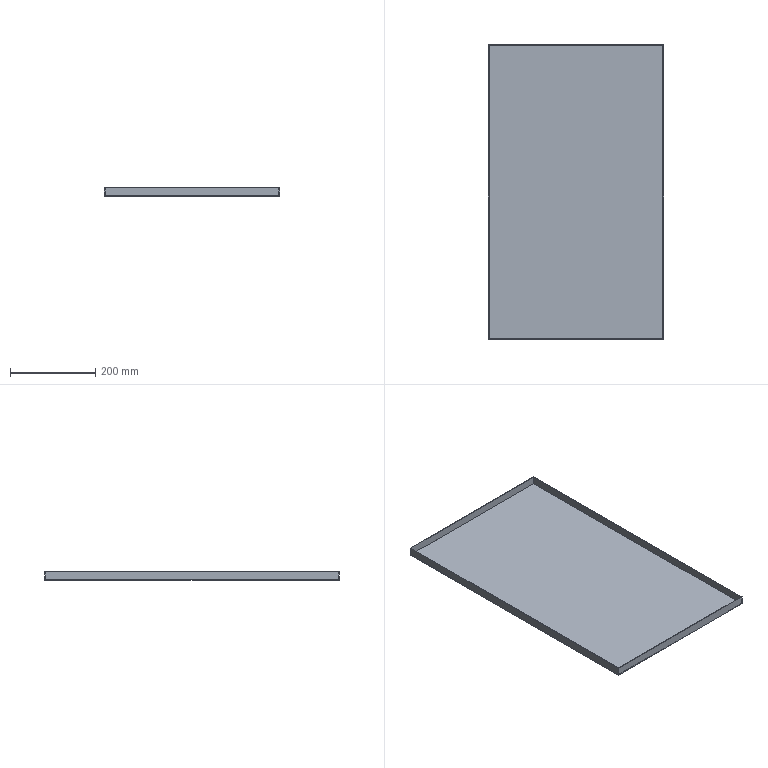Part | STEP file | Lower sealing plate | 1 solid | 11 faces | box 410 x 690 x 20 mm | volume 485234 mm3 | plane 11
STEP:
#1=CARTESIAN_POINT('',(0.,0.,0.));
#2=DIRECTION('',(0.,0.,1.));
#3=DIRECTION('',(1.,0.,0.));
#4=AXIS2_PLACEMENT_3D('',#1,#2,#3);
#5=CARTESIAN_POINT('',(-205.,-345.,0.));
#6=VERTEX_POINT('',#5);
#7=CARTESIAN_POINT('',(205.,-345.,0.));
#8=VERTEX_POINT('',#7);
#9=CARTESIAN_POINT('',(0.,-345.,0.));
#10=DIRECTION('',(1.,0.,0.));
#11=VECTOR('',#10,1.);
#12=LINE('',#9,#11);
#13=CARTESIAN_POINT('',(0.,0.,0.));
#14=DIRECTION('',(0.,0.,1.));
#15=DIRECTION('',(1.,0.,0.));
#16=AXIS2_PLACEMENT_3D('',#13,#14,#15);
#17=PLANE('',#16);
#18=CARTESIAN_POINT('',(0.,-345.));
#19=DIRECTION('',(1.,0.));
#20=VECTOR('',#19,1.);
#21=LINE('',#18,#20);
#22=(GEOMETRIC_REPRESENTATION_CONTEXT(2)PARAMETRIC_REPRESENTATION_CONTEXT()REPRESENTATION_CONTEXT('',''));
#23=DEFINITIONAL_REPRESENTATION('',(#21),#22);
#24=PCURVE('',#17,#23);
#25=CARTESIAN_POINT('',(-205.,-345.,20.));
#26=DIRECTION('',(0.,1.,0.));
#27=DIRECTION('',(0.,0.,1.));
#28=AXIS2_PLACEMENT_3D('',#25,#26,#27);
#29=PLANE('',#28);
#30=CARTESIAN_POINT('',(-20.,205.));
#31=DIRECTION('',(0.,1.));
#32=VECTOR('',#31,1.);
#33=LINE('',#30,#32);
#34=(GEOMETRIC_REPRESENTATION_CONTEXT(2)PARAMETRIC_REPRESENTATION_CONTEXT()REPRESENTATION_CONTEXT('',''));
#35=DEFINITIONAL_REPRESENTATION('',(#33),#34);
#36=PCURVE('',#29,#35);
#37=SURFACE_CURVE('',#12,(#24,#36),.PCURVE_S1.);
#38=EDGE_CURVE('',#6,#8,#37,.T.);
#39=ORIENTED_EDGE('',*,*,#38,.F.);
#40=CARTESIAN_POINT('',(-205.,345.,0.));
#41=VERTEX_POINT('',#40);
#42=CARTESIAN_POINT('',(-205.,0.,0.));
#43=DIRECTION('',(0.,-1.,0.));
#44=VECTOR('',#43,1.);
#45=LINE('',#42,#44);
#46=CARTESIAN_POINT('',(-205.,0.));
#47=DIRECTION('',(0.,-1.));
#48=VECTOR('',#47,1.);
#49=LINE('',#46,#48);
#50=(GEOMETRIC_REPRESENTATION_CONTEXT(2)PARAMETRIC_REPRESENTATION_CONTEXT()REPRESENTATION_CONTEXT('',''));
#51=DEFINITIONAL_REPRESENTATION('',(#49),#50);
#52=PCURVE('',#17,#51);
#53=CARTESIAN_POINT('',(-205.,345.,20.));
#54=DIRECTION('',(1.,0.,0.));
#55=DIRECTION('',(0.,1.,0.));
#56=AXIS2_PLACEMENT_3D('',#53,#54,#55);
#57=PLANE('',#56);
#58=CARTESIAN_POINT('',(-345.,-20.));
#59=DIRECTION('',(-1.,0.));
#60=VECTOR('',#59,1.);
#61=LINE('',#58,#60);
#62=(GEOMETRIC_REPRESENTATION_CONTEXT(2)PARAMETRIC_REPRESENTATION_CONTEXT()REPRESENTATION_CONTEXT('',''));
#63=DEFINITIONAL_REPRESENTATION('',(#61),#62);
#64=PCURVE('',#57,#63);
#65=SURFACE_CURVE('',#45,(#52,#64),.PCURVE_S1.);
#66=EDGE_CURVE('',#41,#6,#65,.T.);
#67=ORIENTED_EDGE('',*,*,#66,.F.);
#68=CARTESIAN_POINT('',(205.,345.,0.));
#69=VERTEX_POINT('',#68);
#70=CARTESIAN_POINT('',(0.,345.,0.));
#71=DIRECTION('',(-1.,0.,0.));
#72=VECTOR('',#71,1.);
#73=LINE('',#70,#72);
#74=CARTESIAN_POINT('',(0.,345.));
#75=DIRECTION('',(-1.,0.));
#76=VECTOR('',#75,1.);
#77=LINE('',#74,#76);
#78=(GEOMETRIC_REPRESENTATION_CONTEXT(2)PARAMETRIC_REPRESENTATION_CONTEXT()REPRESENTATION_CONTEXT('',''));
#79=DEFINITIONAL_REPRESENTATION('',(#77),#78);
#80=PCURVE('',#17,#79);
#81=CARTESIAN_POINT('',(-205.,345.,20.));
#82=DIRECTION('',(0.,-1.,0.));
#83=DIRECTION('',(0.,0.,-1.));
#84=AXIS2_PLACEMENT_3D('',#81,#82,#83);
#85=PLANE('',#84);
#86=CARTESIAN_POINT('',(20.,205.));
#87=DIRECTION('',(0.,-1.));
#88=VECTOR('',#87,1.);
#89=LINE('',#86,#88);
#90=(GEOMETRIC_REPRESENTATION_CONTEXT(2)PARAMETRIC_REPRESENTATION_CONTEXT()REPRESENTATION_CONTEXT('',''));
#91=DEFINITIONAL_REPRESENTATION('',(#89),#90);
#92=PCURVE('',#85,#91);
#93=SURFACE_CURVE('',#73,(#80,#92),.PCURVE_S1.);
#94=EDGE_CURVE('',#69,#41,#93,.T.);
#95=ORIENTED_EDGE('',*,*,#94,.F.);
#96=CARTESIAN_POINT('',(205.,0.,0.));
#97=DIRECTION('',(0.,1.,0.));
#98=VECTOR('',#97,1.);
#99=LINE('',#96,#98);
#100=CARTESIAN_POINT('',(205.,0.));
#101=DIRECTION('',(0.,1.));
#102=VECTOR('',#101,1.);
#103=LINE('',#100,#102);
#104=(GEOMETRIC_REPRESENTATION_CONTEXT(2)PARAMETRIC_REPRESENTATION_CONTEXT()REPRESENTATION_CONTEXT('',''));
#105=DEFINITIONAL_REPRESENTATION('',(#103),#104);
#106=PCURVE('',#17,#105);
#107=CARTESIAN_POINT('',(205.,345.,20.));
#108=DIRECTION('',(-1.,0.,0.));
#109=DIRECTION('',(0.,-1.,0.));
#110=AXIS2_PLACEMENT_3D('',#107,#108,#109);
#111=PLANE('',#110);
#112=CARTESIAN_POINT('',(345.,-20.));
#113=DIRECTION('',(-1.,0.));
#114=VECTOR('',#113,1.);
#115=LINE('',#112,#114);
#116=(GEOMETRIC_REPRESENTATION_CONTEXT(2)PARAMETRIC_REPRESENTATION_CONTEXT()REPRESENTATION_CONTEXT('',''));
#117=DEFINITIONAL_REPRESENTATION('',(#115),#116);
#118=PCURVE('',#111,#117);
#119=SURFACE_CURVE('',#99,(#106,#118),.PCURVE_S1.);
#120=EDGE_CURVE('',#8,#69,#119,.T.);
#121=ORIENTED_EDGE('',*,*,#120,.F.);
#122=EDGE_LOOP('',(#39,#67,#95,#121));
#123=FACE_BOUND('',#122,.T.);
#124=ADVANCED_FACE('',(#123),#17,.F.);
#125=CARTESIAN_POINT('',(205.,345.,20.));
#126=VERTEX_POINT('',#125);
#127=CARTESIAN_POINT('',(205.,345.,20.));
#128=DIRECTION('',(0.,0.,-1.));
#129=VECTOR('',#128,1.);
#130=LINE('',#127,#129);
#131=CARTESIAN_POINT('',(0.,0.));
#132=DIRECTION('',(0.,-1.));
#133=VECTOR('',#132,1.);
#134=LINE('',#131,#133);
#135=(GEOMETRIC_REPRESENTATION_CONTEXT(2)PARAMETRIC_REPRESENTATION_CONTEXT()REPRESENTATION_CONTEXT('',''));
#136=DEFINITIONAL_REPRESENTATION('',(#134),#135);
#137=PCURVE('',#111,#136);
#138=CARTESIAN_POINT('',(0.,410.));
#139=DIRECTION('',(1.,0.));
#140=VECTOR('',#139,1.);
#141=LINE('',#138,#140);
#142=(GEOMETRIC_REPRESENTATION_CONTEXT(2)PARAMETRIC_REPRESENTATION_CONTEXT()REPRESENTATION_CONTEXT('',''));
#143=DEFINITIONAL_REPRESENTATION('',(#141),#142);
#144=PCURVE('',#85,#143);
#145=SURFACE_CURVE('',#130,(#137,#144),.PCURVE_S1.);
#146=EDGE_CURVE('',#126,#69,#145,.T.);
#147=ORIENTED_EDGE('',*,*,#146,.F.);
#148=CARTESIAN_POINT('',(205.,-345.,20.));
#149=VERTEX_POINT('',#148);
#150=CARTESIAN_POINT('',(205.,345.,20.));
#151=DIRECTION('',(0.,1.,0.));
#152=VECTOR('',#151,1.);
#153=LINE('',#150,#152);
#154=CARTESIAN_POINT('',(0.,0.));
#155=DIRECTION('',(-1.,0.));
#156=VECTOR('',#155,1.);
#157=LINE('',#154,#156);
#158=(GEOMETRIC_REPRESENTATION_CONTEXT(2)PARAMETRIC_REPRESENTATION_CONTEXT()REPRESENTATION_CONTEXT('',''));
#159=DEFINITIONAL_REPRESENTATION('',(#157),#158);
#160=PCURVE('',#111,#159);
#161=CARTESIAN_POINT('',(0.,0.,20.));
#162=DIRECTION('',(0.,0.,1.));
#163=DIRECTION('',(1.,0.,0.));
#164=AXIS2_PLACEMENT_3D('',#161,#162,#163);
#165=PLANE('',#164);
#166=CARTESIAN_POINT('',(205.,345.));
#167=DIRECTION('',(0.,1.));
#168=VECTOR('',#167,1.);
#169=LINE('',#166,#168);
#170=(GEOMETRIC_REPRESENTATION_CONTEXT(2)PARAMETRIC_REPRESENTATION_CONTEXT()REPRESENTATION_CONTEXT('',''));
#171=DEFINITIONAL_REPRESENTATION('',(#169),#170);
#172=PCURVE('',#165,#171);
#173=SURFACE_CURVE('',#153,(#160,#172),.PCURVE_S1.);
#174=EDGE_CURVE('',#149,#126,#173,.T.);
#175=ORIENTED_EDGE('',*,*,#174,.F.);
#176=CARTESIAN_POINT('',(205.,-345.,20.));
#177=DIRECTION('',(0.,0.,1.));
#178=VECTOR('',#177,1.);
#179=LINE('',#176,#178);
#180=CARTESIAN_POINT('',(690.,0.));
#181=DIRECTION('',(0.,1.));
#182=VECTOR('',#181,1.);
#183=LINE('',#180,#182);
#184=(GEOMETRIC_REPRESENTATION_CONTEXT(2)PARAMETRIC_REPRESENTATION_CONTEXT()REPRESENTATION_CONTEXT('',''));
#185=DEFINITIONAL_REPRESENTATION('',(#183),#184);
#186=PCURVE('',#111,#185);
#187=CARTESIAN_POINT('',(0.,410.));
#188=DIRECTION('',(1.,0.));
#189=VECTOR('',#188,1.);
#190=LINE('',#187,#189);
#191=(GEOMETRIC_REPRESENTATION_CONTEXT(2)PARAMETRIC_REPRESENTATION_CONTEXT()REPRESENTATION_CONTEXT('',''));
#192=DEFINITIONAL_REPRESENTATION('',(#190),#191);
#193=PCURVE('',#29,#192);
#194=SURFACE_CURVE('',#179,(#186,#193),.PCURVE_S1.);
#195=EDGE_CURVE('',#8,#149,#194,.T.);
#196=ORIENTED_EDGE('',*,*,#195,.F.);
#197=ORIENTED_EDGE('',*,*,#120,.T.);
#198=EDGE_LOOP('',(#147,#175,#196,#197));
#199=FACE_BOUND('',#198,.T.);
#200=ADVANCED_FACE('',(#199),#111,.F.);
#201=ORIENTED_EDGE('',*,*,#195,.T.);
#202=CARTESIAN_POINT('',(-205.,-345.,20.));
#203=VERTEX_POINT('',#202);
#204=CARTESIAN_POINT('',(-205.,-345.,20.));
#205=DIRECTION('',(1.,0.,0.));
#206=VECTOR('',#205,1.);
#207=LINE('',#204,#206);
#208=CARTESIAN_POINT('',(0.,0.));
#209=DIRECTION('',(0.,1.));
#210=VECTOR('',#209,1.);
#211=LINE('',#208,#210);
#212=(GEOMETRIC_REPRESENTATION_CONTEXT(2)PARAMETRIC_REPRESENTATION_CONTEXT()REPRESENTATION_CONTEXT('',''));
#213=DEFINITIONAL_REPRESENTATION('',(#211),#212);
#214=PCURVE('',#29,#213);
#215=CARTESIAN_POINT('',(-205.,-345.));
#216=DIRECTION('',(1.,0.));
#217=VECTOR('',#216,1.);
#218=LINE('',#215,#217);
#219=(GEOMETRIC_REPRESENTATION_CONTEXT(2)PARAMETRIC_REPRESENTATION_CONTEXT()REPRESENTATION_CONTEXT('',''));
#220=DEFINITIONAL_REPRESENTATION('',(#218),#219);
#221=PCURVE('',#165,#220);
#222=SURFACE_CURVE('',#207,(#214,#221),.PCURVE_S1.);
#223=EDGE_CURVE('',#203,#149,#222,.T.);
#224=ORIENTED_EDGE('',*,*,#223,.F.);
#225=CARTESIAN_POINT('',(-205.,-345.,20.));
#226=DIRECTION('',(0.,0.,1.));
#227=VECTOR('',#226,1.);
#228=LINE('',#225,#227);
#229=CARTESIAN_POINT('',(0.,0.));
#230=DIRECTION('',(1.,0.));
#231=VECTOR('',#230,1.);
#232=LINE('',#229,#231);
#233=(GEOMETRIC_REPRESENTATION_CONTEXT(2)PARAMETRIC_REPRESENTATION_CONTEXT()REPRESENTATION_CONTEXT('',''));
#234=DEFINITIONAL_REPRESENTATION('',(#232),#233);
#235=PCURVE('',#29,#234);
#236=CARTESIAN_POINT('',(-690.,0.));
#237=DIRECTION('',(0.,1.));
#238=VECTOR('',#237,1.);
#239=LINE('',#236,#238);
#240=(GEOMETRIC_REPRESENTATION_CONTEXT(2)PARAMETRIC_REPRESENTATION_CONTEXT()REPRESENTATION_CONTEXT('',''));
#241=DEFINITIONAL_REPRESENTATION('',(#239),#240);
#242=PCURVE('',#57,#241);
#243=SURFACE_CURVE('',#228,(#235,#242),.PCURVE_S1.);
#244=EDGE_CURVE('',#6,#203,#243,.T.);
#245=ORIENTED_EDGE('',*,*,#244,.F.);
#246=ORIENTED_EDGE('',*,*,#38,.T.);
#247=EDGE_LOOP('',(#201,#224,#245,#246));
#248=FACE_BOUND('',#247,.T.);
#249=ADVANCED_FACE('',(#248),#29,.F.);
#250=ORIENTED_EDGE('',*,*,#244,.T.);
#251=CARTESIAN_POINT('',(-205.,345.,20.));
#252=VERTEX_POINT('',#251);
#253=CARTESIAN_POINT('',(-205.,345.,20.));
#254=DIRECTION('',(0.,-1.,0.));
#255=VECTOR('',#254,1.);
#256=LINE('',#253,#255);
#257=CARTESIAN_POINT('',(0.,0.));
#258=DIRECTION('',(-1.,0.));
#259=VECTOR('',#258,1.);
#260=LINE('',#257,#259);
#261=(GEOMETRIC_REPRESENTATION_CONTEXT(2)PARAMETRIC_REPRESENTATION_CONTEXT()REPRESENTATION_CONTEXT('',''));
#262=DEFINITIONAL_REPRESENTATION('',(#260),#261);
#263=PCURVE('',#57,#262);
#264=CARTESIAN_POINT('',(-205.,345.));
#265=DIRECTION('',(0.,-1.));
#266=VECTOR('',#265,1.);
#267=LINE('',#264,#266);
#268=(GEOMETRIC_REPRESENTATION_CONTEXT(2)PARAMETRIC_REPRESENTATION_CONTEXT()REPRESENTATION_CONTEXT('',''));
#269=DEFINITIONAL_REPRESENTATION('',(#267),#268);
#270=PCURVE('',#165,#269);
#271=SURFACE_CURVE('',#256,(#263,#270),.PCURVE_S1.);
#272=EDGE_CURVE('',#252,#203,#271,.T.);
#273=ORIENTED_EDGE('',*,*,#272,.F.);
#274=CARTESIAN_POINT('',(-205.,345.,20.));
#275=DIRECTION('',(0.,0.,1.));
#276=VECTOR('',#275,1.);
#277=LINE('',#274,#276);
#278=CARTESIAN_POINT('',(0.,0.));
#279=DIRECTION('',(0.,1.));
#280=VECTOR('',#279,1.);
#281=LINE('',#278,#280);
#282=(GEOMETRIC_REPRESENTATION_CONTEXT(2)PARAMETRIC_REPRESENTATION_CONTEXT()REPRESENTATION_CONTEXT('',''));
#283=DEFINITIONAL_REPRESENTATION('',(#281),#282);
#284=PCURVE('',#57,#283);
#285=CARTESIAN_POINT('',(0.,0.));
#286=DIRECTION('',(-1.,0.));
#287=VECTOR('',#286,1.);
#288=LINE('',#285,#287);
#289=(GEOMETRIC_REPRESENTATION_CONTEXT(2)PARAMETRIC_REPRESENTATION_CONTEXT()REPRESENTATION_CONTEXT('',''));
#290=DEFINITIONAL_REPRESENTATION('',(#288),#289);
#291=PCURVE('',#85,#290);
#292=SURFACE_CURVE('',#277,(#284,#291),.PCURVE_S1.);
#293=EDGE_CURVE('',#41,#252,#292,.T.);
#294=ORIENTED_EDGE('',*,*,#293,.F.);
#295=ORIENTED_EDGE('',*,*,#66,.T.);
#296=EDGE_LOOP('',(#250,#273,#294,#295));
#297=FACE_BOUND('',#296,.T.);
#298=ADVANCED_FACE('',(#297),#57,.F.);
#299=ORIENTED_EDGE('',*,*,#293,.T.);
#300=CARTESIAN_POINT('',(-205.,345.,20.));
#301=DIRECTION('',(-1.,0.,0.));
#302=VECTOR('',#301,1.);
#303=LINE('',#300,#302);
#304=CARTESIAN_POINT('',(0.,0.));
#305=DIRECTION('',(0.,-1.));
#306=VECTOR('',#305,1.);
#307=LINE('',#304,#306);
#308=(GEOMETRIC_REPRESENTATION_CONTEXT(2)PARAMETRIC_REPRESENTATION_CONTEXT()REPRESENTATION_CONTEXT('',''));
#309=DEFINITIONAL_REPRESENTATION('',(#307),#308);
#310=PCURVE('',#85,#309);
#311=CARTESIAN_POINT('',(-205.,345.));
#312=DIRECTION('',(-1.,0.));
#313=VECTOR('',#312,1.);
#314=LINE('',#311,#313);
#315=(GEOMETRIC_REPRESENTATION_CONTEXT(2)PARAMETRIC_REPRESENTATION_CONTEXT()REPRESENTATION_CONTEXT('',''));
#316=DEFINITIONAL_REPRESENTATION('',(#314),#315);
#317=PCURVE('',#165,#316);
#318=SURFACE_CURVE('',#303,(#310,#317),.PCURVE_S1.);
#319=EDGE_CURVE('',#126,#252,#318,.T.);
#320=ORIENTED_EDGE('',*,*,#319,.F.);
#321=ORIENTED_EDGE('',*,*,#146,.T.);
#322=ORIENTED_EDGE('',*,*,#94,.T.);
#323=EDGE_LOOP('',(#299,#320,#321,#322));
#324=FACE_BOUND('',#323,.T.);
#325=ADVANCED_FACE('',(#324),#85,.F.);
#326=ORIENTED_EDGE('',*,*,#272,.T.);
#327=ORIENTED_EDGE('',*,*,#223,.T.);
#328=ORIENTED_EDGE('',*,*,#174,.T.);
#329=ORIENTED_EDGE('',*,*,#319,.T.);
#330=EDGE_LOOP('',(#326,#327,#328,#329));
#331=FACE_BOUND('',#330,.T.);
#332=CARTESIAN_POINT('',(-203.5,-343.5,20.));
#333=VERTEX_POINT('',#332);
#334=CARTESIAN_POINT('',(-203.5,343.5,20.));
#335=VERTEX_POINT('',#334);
#336=CARTESIAN_POINT('',(-203.5,0.,20.));
#337=DIRECTION('',(0.,1.,0.));
#338=VECTOR('',#337,1.);
#339=LINE('',#336,#338);
#340=CARTESIAN_POINT('',(-203.5,0.));
#341=DIRECTION('',(0.,1.));
#342=VECTOR('',#341,1.);
#343=LINE('',#340,#342);
#344=(GEOMETRIC_REPRESENTATION_CONTEXT(2)PARAMETRIC_REPRESENTATION_CONTEXT()REPRESENTATION_CONTEXT('',''));
#345=DEFINITIONAL_REPRESENTATION('',(#343),#344);
#346=PCURVE('',#165,#345);
#347=CARTESIAN_POINT('',(-203.5,345.,20.));
#348=DIRECTION('',(1.,0.,0.));
#349=DIRECTION('',(0.,1.,0.));
#350=AXIS2_PLACEMENT_3D('',#347,#348,#349);
#351=PLANE('',#350);
#352=CARTESIAN_POINT('',(-345.,0.));
#353=DIRECTION('',(1.,0.));
#354=VECTOR('',#353,1.);
#355=LINE('',#352,#354);
#356=(GEOMETRIC_REPRESENTATION_CONTEXT(2)PARAMETRIC_REPRESENTATION_CONTEXT()REPRESENTATION_CONTEXT('',''));
#357=DEFINITIONAL_REPRESENTATION('',(#355),#356);
#358=PCURVE('',#351,#357);
#359=SURFACE_CURVE('',#339,(#346,#358),.PCURVE_S1.);
#360=EDGE_CURVE('',#333,#335,#359,.T.);
#361=ORIENTED_EDGE('',*,*,#360,.T.);
#362=CARTESIAN_POINT('',(203.5,343.5,20.));
#363=VERTEX_POINT('',#362);
#364=CARTESIAN_POINT('',(0.,343.5,20.));
#365=DIRECTION('',(1.,0.,0.));
#366=VECTOR('',#365,1.);
#367=LINE('',#364,#366);
#368=CARTESIAN_POINT('',(0.,343.5));
#369=DIRECTION('',(1.,0.));
#370=VECTOR('',#369,1.);
#371=LINE('',#368,#370);
#372=(GEOMETRIC_REPRESENTATION_CONTEXT(2)PARAMETRIC_REPRESENTATION_CONTEXT()REPRESENTATION_CONTEXT('',''));
#373=DEFINITIONAL_REPRESENTATION('',(#371),#372);
#374=PCURVE('',#165,#373);
#375=CARTESIAN_POINT('',(-205.,343.5,20.));
#376=DIRECTION('',(0.,-1.,0.));
#377=DIRECTION('',(0.,0.,-1.));
#378=AXIS2_PLACEMENT_3D('',#375,#376,#377);
#379=PLANE('',#378);
#380=CARTESIAN_POINT('',(0.,205.));
#381=DIRECTION('',(0.,1.));
#382=VECTOR('',#381,1.);
#383=LINE('',#380,#382);
#384=(GEOMETRIC_REPRESENTATION_CONTEXT(2)PARAMETRIC_REPRESENTATION_CONTEXT()REPRESENTATION_CONTEXT('',''));
#385=DEFINITIONAL_REPRESENTATION('',(#383),#384);
#386=PCURVE('',#379,#385);
#387=SURFACE_CURVE('',#367,(#374,#386),.PCURVE_S1.);
#388=EDGE_CURVE('',#335,#363,#387,.T.);
#389=ORIENTED_EDGE('',*,*,#388,.T.);
#390=CARTESIAN_POINT('',(203.5,-343.5,20.));
#391=VERTEX_POINT('',#390);
#392=CARTESIAN_POINT('',(203.5,0.,20.));
#393=DIRECTION('',(0.,-1.,0.));
#394=VECTOR('',#393,1.);
#395=LINE('',#392,#394);
#396=CARTESIAN_POINT('',(203.5,0.));
#397=DIRECTION('',(0.,-1.));
#398=VECTOR('',#397,1.);
#399=LINE('',#396,#398);
#400=(GEOMETRIC_REPRESENTATION_CONTEXT(2)PARAMETRIC_REPRESENTATION_CONTEXT()REPRESENTATION_CONTEXT('',''));
#401=DEFINITIONAL_REPRESENTATION('',(#399),#400);
#402=PCURVE('',#165,#401);
#403=CARTESIAN_POINT('',(203.5,345.,20.));
#404=DIRECTION('',(-1.,0.,0.));
#405=DIRECTION('',(0.,-1.,0.));
#406=AXIS2_PLACEMENT_3D('',#403,#404,#405);
#407=PLANE('',#406);
#408=CARTESIAN_POINT('',(345.,0.));
#409=DIRECTION('',(1.,0.));
#410=VECTOR('',#409,1.);
#411=LINE('',#408,#410);
#412=(GEOMETRIC_REPRESENTATION_CONTEXT(2)PARAMETRIC_REPRESENTATION_CONTEXT()REPRESENTATION_CONTEXT('',''));
#413=DEFINITIONAL_REPRESENTATION('',(#411),#412);
#414=PCURVE('',#407,#413);
#415=SURFACE_CURVE('',#395,(#402,#414),.PCURVE_S1.);
#416=EDGE_CURVE('',#363,#391,#415,.T.);
#417=ORIENTED_EDGE('',*,*,#416,.T.);
#418=CARTESIAN_POINT('',(0.,-343.5,20.));
#419=DIRECTION('',(-1.,0.,0.));
#420=VECTOR('',#419,1.);
#421=LINE('',#418,#420);
#422=CARTESIAN_POINT('',(0.,-343.5));
#423=DIRECTION('',(-1.,0.));
#424=VECTOR('',#423,1.);
#425=LINE('',#422,#424);
#426=(GEOMETRIC_REPRESENTATION_CONTEXT(2)PARAMETRIC_REPRESENTATION_CONTEXT()REPRESENTATION_CONTEXT('',''));
#427=DEFINITIONAL_REPRESENTATION('',(#425),#426);
#428=PCURVE('',#165,#427);
#429=CARTESIAN_POINT('',(-205.,-343.5,20.));
#430=DIRECTION('',(0.,1.,0.));
#431=DIRECTION('',(0.,0.,1.));
#432=AXIS2_PLACEMENT_3D('',#429,#430,#431);
#433=PLANE('',#432);
#434=CARTESIAN_POINT('',(0.,205.));
#435=DIRECTION('',(0.,-1.));
#436=VECTOR('',#435,1.);
#437=LINE('',#434,#436);
#438=(GEOMETRIC_REPRESENTATION_CONTEXT(2)PARAMETRIC_REPRESENTATION_CONTEXT()REPRESENTATION_CONTEXT('',''));
#439=DEFINITIONAL_REPRESENTATION('',(#437),#438);
#440=PCURVE('',#433,#439);
#441=SURFACE_CURVE('',#421,(#428,#440),.PCURVE_S1.);
#442=EDGE_CURVE('',#391,#333,#441,.T.);
#443=ORIENTED_EDGE('',*,*,#442,.T.);
#444=EDGE_LOOP('',(#361,#389,#417,#443));
#445=FACE_BOUND('',#444,.T.);
#446=ADVANCED_FACE('',(#331,#445),#165,.T.);
#447=ORIENTED_EDGE('',*,*,#388,.F.);
#448=CARTESIAN_POINT('',(-203.5,343.5,1.5));
#449=VERTEX_POINT('',#448);
#450=CARTESIAN_POINT('',(-203.5,343.5,20.));
#451=DIRECTION('',(0.,0.,-1.));
#452=VECTOR('',#451,1.);
#453=LINE('',#450,#452);
#454=CARTESIAN_POINT('',(0.,1.5));
#455=DIRECTION('',(1.,0.));
#456=VECTOR('',#455,1.);
#457=LINE('',#454,#456);
#458=(GEOMETRIC_REPRESENTATION_CONTEXT(2)PARAMETRIC_REPRESENTATION_CONTEXT()REPRESENTATION_CONTEXT('',''));
#459=DEFINITIONAL_REPRESENTATION('',(#457),#458);
#460=PCURVE('',#379,#459);
#461=CARTESIAN_POINT('',(-1.5,0.));
#462=DIRECTION('',(0.,-1.));
#463=VECTOR('',#462,1.);
#464=LINE('',#461,#463);
#465=(GEOMETRIC_REPRESENTATION_CONTEXT(2)PARAMETRIC_REPRESENTATION_CONTEXT()REPRESENTATION_CONTEXT('',''));
#466=DEFINITIONAL_REPRESENTATION('',(#464),#465);
#467=PCURVE('',#351,#466);
#468=SURFACE_CURVE('',#453,(#460,#467),.PCURVE_S1.);
#469=EDGE_CURVE('',#335,#449,#468,.T.);
#470=ORIENTED_EDGE('',*,*,#469,.T.);
#471=CARTESIAN_POINT('',(203.5,343.5,1.5));
#472=VERTEX_POINT('',#471);
#473=CARTESIAN_POINT('',(-205.,343.5,1.5));
#474=DIRECTION('',(1.,0.,0.));
#475=VECTOR('',#474,1.);
#476=LINE('',#473,#475);
#477=CARTESIAN_POINT('',(18.5,0.));
#478=DIRECTION('',(0.,1.));
#479=VECTOR('',#478,1.);
#480=LINE('',#477,#479);
#481=(GEOMETRIC_REPRESENTATION_CONTEXT(2)PARAMETRIC_REPRESENTATION_CONTEXT()REPRESENTATION_CONTEXT('',''));
#482=DEFINITIONAL_REPRESENTATION('',(#480),#481);
#483=PCURVE('',#379,#482);
#484=CARTESIAN_POINT('',(0.,0.,1.5));
#485=DIRECTION('',(0.,0.,1.));
#486=DIRECTION('',(1.,0.,0.));
#487=AXIS2_PLACEMENT_3D('',#484,#485,#486);
#488=PLANE('',#487);
#489=CARTESIAN_POINT('',(-205.,343.5));
#490=DIRECTION('',(1.,0.));
#491=VECTOR('',#490,1.);
#492=LINE('',#489,#491);
#493=(GEOMETRIC_REPRESENTATION_CONTEXT(2)PARAMETRIC_REPRESENTATION_CONTEXT()REPRESENTATION_CONTEXT('',''));
#494=DEFINITIONAL_REPRESENTATION('',(#492),#493);
#495=PCURVE('',#488,#494);
#496=SURFACE_CURVE('',#476,(#483,#495),.PCURVE_S1.);
#497=EDGE_CURVE('',#449,#472,#496,.T.);
#498=ORIENTED_EDGE('',*,*,#497,.T.);
#499=CARTESIAN_POINT('',(203.5,343.5,20.));
#500=DIRECTION('',(0.,0.,1.));
#501=VECTOR('',#500,1.);
#502=LINE('',#499,#501);
#503=CARTESIAN_POINT('',(0.,408.5));
#504=DIRECTION('',(-1.,0.));
#505=VECTOR('',#504,1.);
#506=LINE('',#503,#505);
#507=(GEOMETRIC_REPRESENTATION_CONTEXT(2)PARAMETRIC_REPRESENTATION_CONTEXT()REPRESENTATION_CONTEXT('',''));
#508=DEFINITIONAL_REPRESENTATION('',(#506),#507);
#509=PCURVE('',#379,#508);
#510=CARTESIAN_POINT('',(1.5,0.));
#511=DIRECTION('',(0.,1.));
#512=VECTOR('',#511,1.);
#513=LINE('',#510,#512);
#514=(GEOMETRIC_REPRESENTATION_CONTEXT(2)PARAMETRIC_REPRESENTATION_CONTEXT()REPRESENTATION_CONTEXT('',''));
#515=DEFINITIONAL_REPRESENTATION('',(#513),#514);
#516=PCURVE('',#407,#515);
#517=SURFACE_CURVE('',#502,(#509,#516),.PCURVE_S1.);
#518=EDGE_CURVE('',#472,#363,#517,.T.);
#519=ORIENTED_EDGE('',*,*,#518,.T.);
#520=EDGE_LOOP('',(#447,#470,#498,#519));
#521=FACE_BOUND('',#520,.T.);
#522=ADVANCED_FACE('',(#521),#379,.T.);
#523=ORIENTED_EDGE('',*,*,#360,.F.);
#524=CARTESIAN_POINT('',(-203.5,-343.5,1.5));
#525=VERTEX_POINT('',#524);
#526=CARTESIAN_POINT('',(-203.5,-343.5,20.));
#527=DIRECTION('',(0.,0.,-1.));
#528=VECTOR('',#527,1.);
#529=LINE('',#526,#528);
#530=CARTESIAN_POINT('',(-688.5,0.));
#531=DIRECTION('',(0.,-1.));
#532=VECTOR('',#531,1.);
#533=LINE('',#530,#532);
#534=(GEOMETRIC_REPRESENTATION_CONTEXT(2)PARAMETRIC_REPRESENTATION_CONTEXT()REPRESENTATION_CONTEXT('',''));
#535=DEFINITIONAL_REPRESENTATION('',(#533),#534);
#536=PCURVE('',#351,#535);
#537=CARTESIAN_POINT('',(0.,1.5));
#538=DIRECTION('',(-1.,0.));
#539=VECTOR('',#538,1.);
#540=LINE('',#537,#539);
#541=(GEOMETRIC_REPRESENTATION_CONTEXT(2)PARAMETRIC_REPRESENTATION_CONTEXT()REPRESENTATION_CONTEXT('',''));
#542=DEFINITIONAL_REPRESENTATION('',(#540),#541);
#543=PCURVE('',#433,#542);
#544=SURFACE_CURVE('',#529,(#536,#543),.PCURVE_S1.);
#545=EDGE_CURVE('',#333,#525,#544,.T.);
#546=ORIENTED_EDGE('',*,*,#545,.T.);
#547=CARTESIAN_POINT('',(-203.5,345.,1.5));
#548=DIRECTION('',(0.,1.,0.));
#549=VECTOR('',#548,1.);
#550=LINE('',#547,#549);
#551=CARTESIAN_POINT('',(0.,-18.5));
#552=DIRECTION('',(1.,0.));
#553=VECTOR('',#552,1.);
#554=LINE('',#551,#553);
#555=(GEOMETRIC_REPRESENTATION_CONTEXT(2)PARAMETRIC_REPRESENTATION_CONTEXT()REPRESENTATION_CONTEXT('',''));
#556=DEFINITIONAL_REPRESENTATION('',(#554),#555);
#557=PCURVE('',#351,#556);
#558=CARTESIAN_POINT('',(-203.5,345.));
#559=DIRECTION('',(0.,1.));
#560=VECTOR('',#559,1.);
#561=LINE('',#558,#560);
#562=(GEOMETRIC_REPRESENTATION_CONTEXT(2)PARAMETRIC_REPRESENTATION_CONTEXT()REPRESENTATION_CONTEXT('',''));
#563=DEFINITIONAL_REPRESENTATION('',(#561),#562);
#564=PCURVE('',#488,#563);
#565=SURFACE_CURVE('',#550,(#557,#564),.PCURVE_S1.);
#566=EDGE_CURVE('',#525,#449,#565,.T.);
#567=ORIENTED_EDGE('',*,*,#566,.T.);
#568=ORIENTED_EDGE('',*,*,#469,.F.);
#569=EDGE_LOOP('',(#523,#546,#567,#568));
#570=FACE_BOUND('',#569,.T.);
#571=ADVANCED_FACE('',(#570),#351,.T.);
#572=ORIENTED_EDGE('',*,*,#442,.F.);
#573=CARTESIAN_POINT('',(203.5,-343.5,1.5));
#574=VERTEX_POINT('',#573);
#575=CARTESIAN_POINT('',(203.5,-343.5,20.));
#576=DIRECTION('',(0.,0.,-1.));
#577=VECTOR('',#576,1.);
#578=LINE('',#575,#577);
#579=CARTESIAN_POINT('',(0.,408.5));
#580=DIRECTION('',(-1.,0.));
#581=VECTOR('',#580,1.);
#582=LINE('',#579,#581);
#583=(GEOMETRIC_REPRESENTATION_CONTEXT(2)PARAMETRIC_REPRESENTATION_CONTEXT()REPRESENTATION_CONTEXT('',''));
#584=DEFINITIONAL_REPRESENTATION('',(#582),#583);
#585=PCURVE('',#433,#584);
#586=CARTESIAN_POINT('',(688.5,0.));
#587=DIRECTION('',(0.,-1.));
#588=VECTOR('',#587,1.);
#589=LINE('',#586,#588);
#590=(GEOMETRIC_REPRESENTATION_CONTEXT(2)PARAMETRIC_REPRESENTATION_CONTEXT()REPRESENTATION_CONTEXT('',''));
#591=DEFINITIONAL_REPRESENTATION('',(#589),#590);
#592=PCURVE('',#407,#591);
#593=SURFACE_CURVE('',#578,(#585,#592),.PCURVE_S1.);
#594=EDGE_CURVE('',#391,#574,#593,.T.);
#595=ORIENTED_EDGE('',*,*,#594,.T.);
#596=CARTESIAN_POINT('',(-205.,-343.5,1.5));
#597=DIRECTION('',(-1.,0.,0.));
#598=VECTOR('',#597,1.);
#599=LINE('',#596,#598);
#600=CARTESIAN_POINT('',(-18.5,0.));
#601=DIRECTION('',(0.,-1.));
#602=VECTOR('',#601,1.);
#603=LINE('',#600,#602);
#604=(GEOMETRIC_REPRESENTATION_CONTEXT(2)PARAMETRIC_REPRESENTATION_CONTEXT()REPRESENTATION_CONTEXT('',''));
#605=DEFINITIONAL_REPRESENTATION('',(#603),#604);
#606=PCURVE('',#433,#605);
#607=CARTESIAN_POINT('',(-205.,-343.5));
#608=DIRECTION('',(-1.,0.));
#609=VECTOR('',#608,1.);
#610=LINE('',#607,#609);
#611=(GEOMETRIC_REPRESENTATION_CONTEXT(2)PARAMETRIC_REPRESENTATION_CONTEXT()REPRESENTATION_CONTEXT('',''));
#612=DEFINITIONAL_REPRESENTATION('',(#610),#611);
#613=PCURVE('',#488,#612);
#614=SURFACE_CURVE('',#599,(#606,#613),.PCURVE_S1.);
#615=EDGE_CURVE('',#574,#525,#614,.T.);
#616=ORIENTED_EDGE('',*,*,#615,.T.);
#617=ORIENTED_EDGE('',*,*,#545,.F.);
#618=EDGE_LOOP('',(#572,#595,#616,#617));
#619=FACE_BOUND('',#618,.T.);
#620=ADVANCED_FACE('',(#619),#433,.T.);
#621=ORIENTED_EDGE('',*,*,#416,.F.);
#622=ORIENTED_EDGE('',*,*,#518,.F.);
#623=CARTESIAN_POINT('',(203.5,345.,1.5));
#624=DIRECTION('',(0.,-1.,0.));
#625=VECTOR('',#624,1.);
#626=LINE('',#623,#625);
#627=CARTESIAN_POINT('',(0.,-18.5));
#628=DIRECTION('',(1.,0.));
#629=VECTOR('',#628,1.);
#630=LINE('',#627,#629);
#631=(GEOMETRIC_REPRESENTATION_CONTEXT(2)PARAMETRIC_REPRESENTATION_CONTEXT()REPRESENTATION_CONTEXT('',''));
#632=DEFINITIONAL_REPRESENTATION('',(#630),#631);
#633=PCURVE('',#407,#632);
#634=CARTESIAN_POINT('',(203.5,345.));
#635=DIRECTION('',(0.,-1.));
#636=VECTOR('',#635,1.);
#637=LINE('',#634,#636);
#638=(GEOMETRIC_REPRESENTATION_CONTEXT(2)PARAMETRIC_REPRESENTATION_CONTEXT()REPRESENTATION_CONTEXT('',''));
#639=DEFINITIONAL_REPRESENTATION('',(#637),#638);
#640=PCURVE('',#488,#639);
#641=SURFACE_CURVE('',#626,(#633,#640),.PCURVE_S1.);
#642=EDGE_CURVE('',#472,#574,#641,.T.);
#643=ORIENTED_EDGE('',*,*,#642,.T.);
#644=ORIENTED_EDGE('',*,*,#594,.F.);
#645=EDGE_LOOP('',(#621,#622,#643,#644));
#646=FACE_BOUND('',#645,.T.);
#647=ADVANCED_FACE('',(#646),#407,.T.);
#648=ORIENTED_EDGE('',*,*,#566,.F.);
#649=ORIENTED_EDGE('',*,*,#615,.F.);
#650=ORIENTED_EDGE('',*,*,#642,.F.);
#651=ORIENTED_EDGE('',*,*,#497,.F.);
#652=EDGE_LOOP('',(#648,#649,#650,#651));
#653=FACE_BOUND('',#652,.T.);
#654=ADVANCED_FACE('',(#653),#488,.T.);
#655=CLOSED_SHELL('',(#124,#200,#249,#298,#325,#446,#522,#571,#620,#647,#654));
#656=MANIFOLD_SOLID_BREP('',#655);
#657=(LENGTH_UNIT()NAMED_UNIT(*)SI_UNIT(.MILLI.,.METRE.));
#658=UNCERTAINTY_MEASURE_WITH_UNIT(LENGTH_MEASURE(0.0000001),#657,'','');
#659=(NAMED_UNIT(*)PLANE_ANGLE_UNIT()SI_UNIT($,.RADIAN.));
#660=(NAMED_UNIT(*)SI_UNIT($,.STERADIAN.)SOLID_ANGLE_UNIT());
#661=(GEOMETRIC_REPRESENTATION_CONTEXT(3)GLOBAL_UNCERTAINTY_ASSIGNED_CONTEXT((#658))GLOBAL_UNIT_ASSIGNED_CONTEXT((#657,#659,#660))REPRESENTATION_CONTEXT('',''));
#662=ADVANCED_BREP_SHAPE_REPRESENTATION('',(#4,#656),#661);